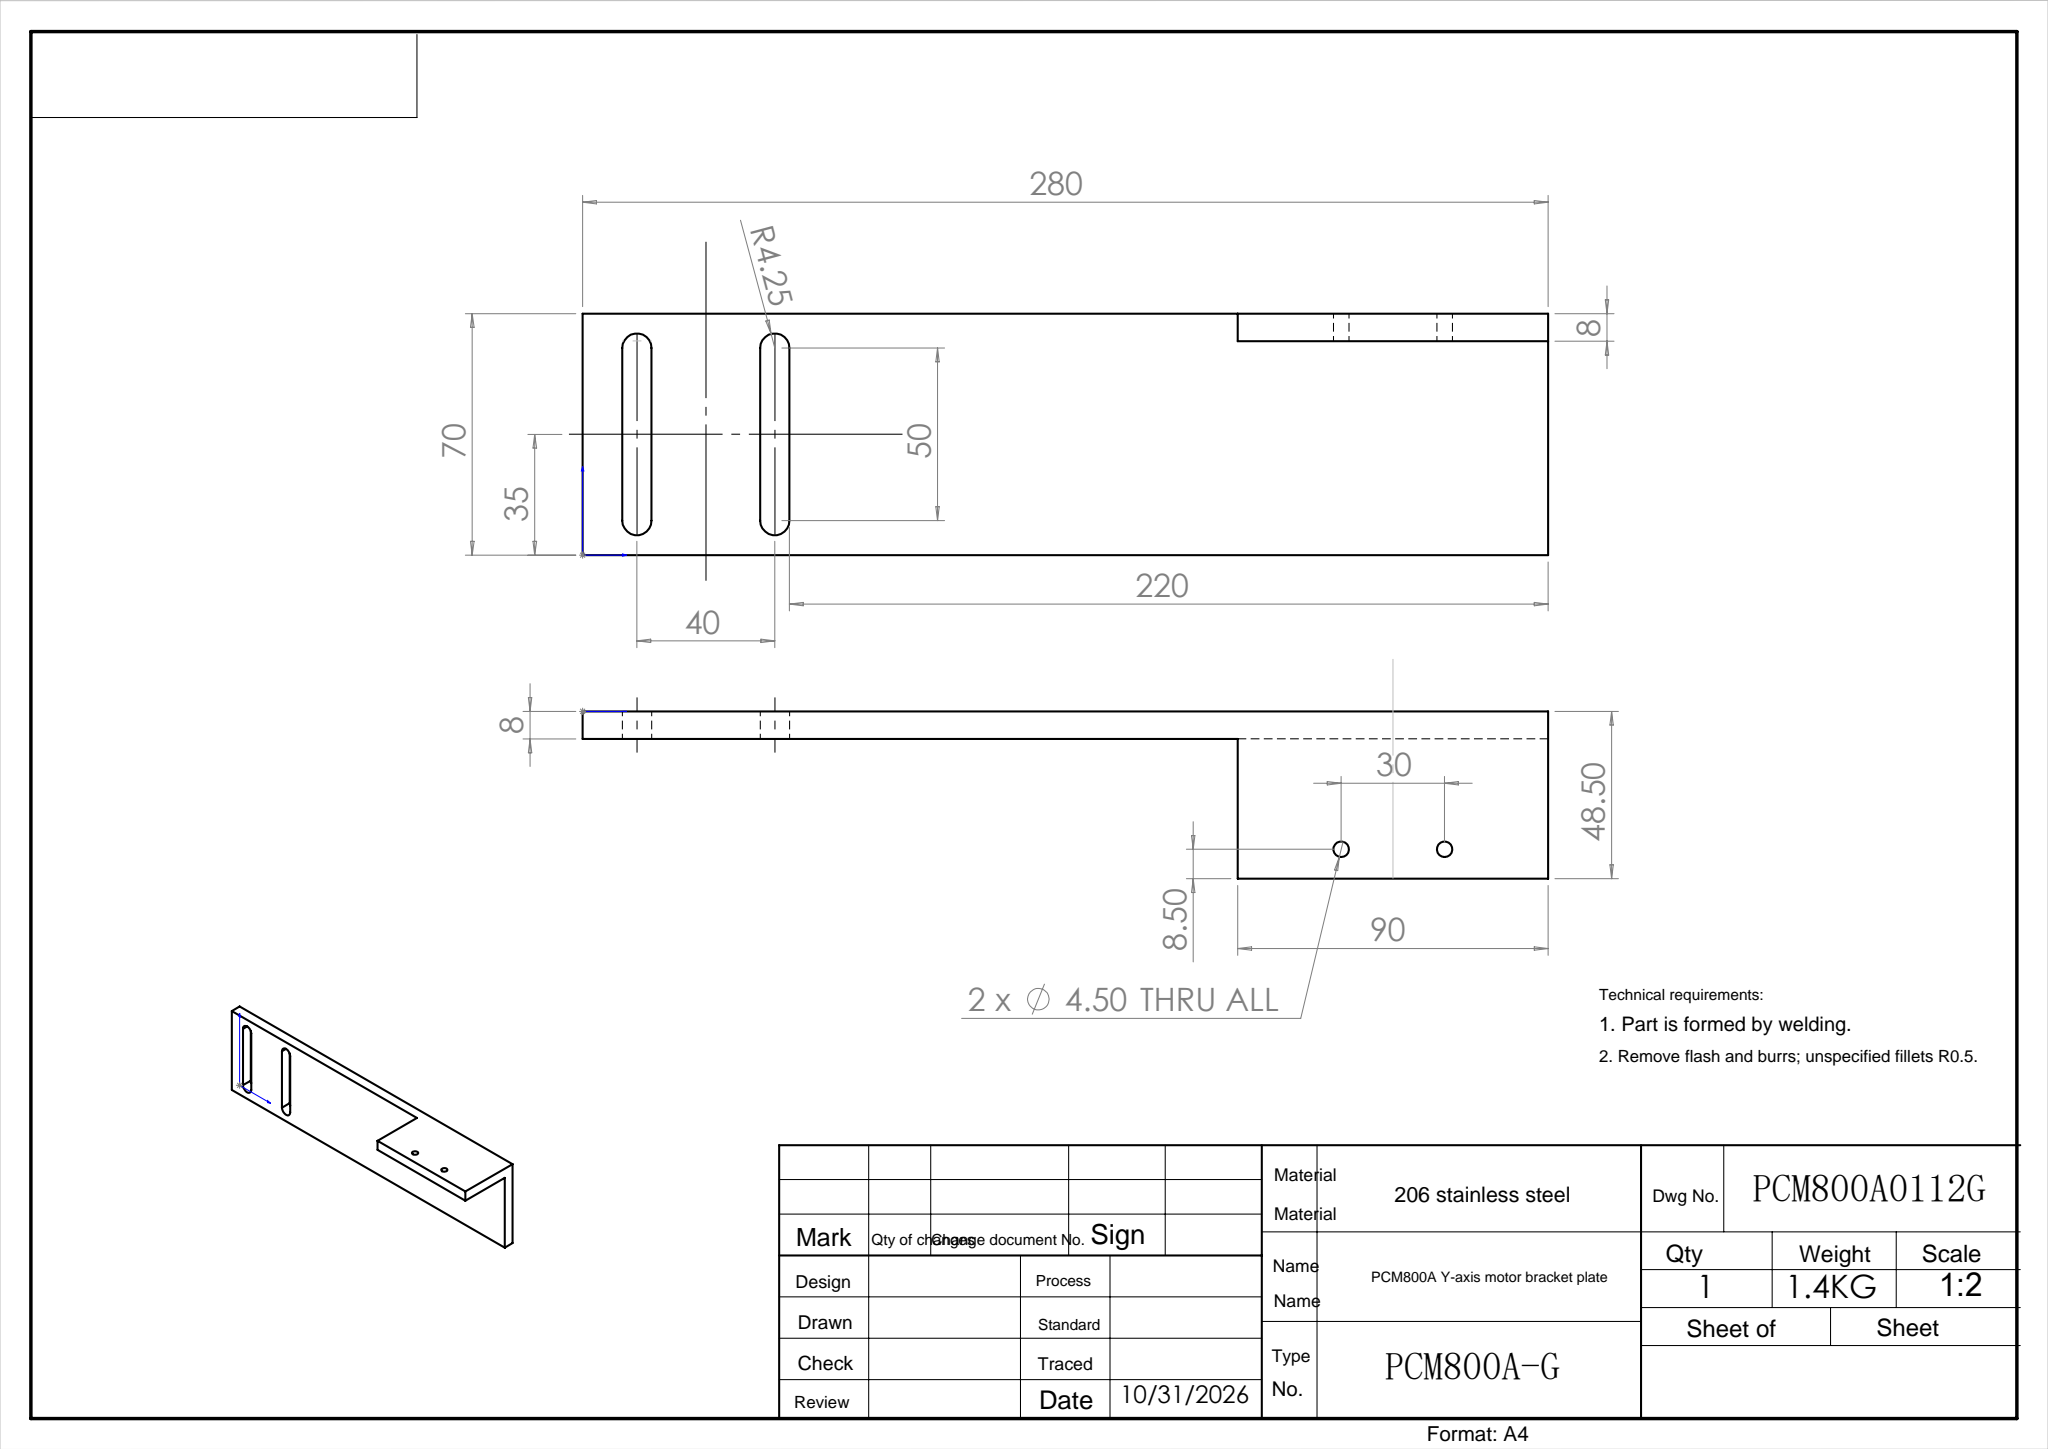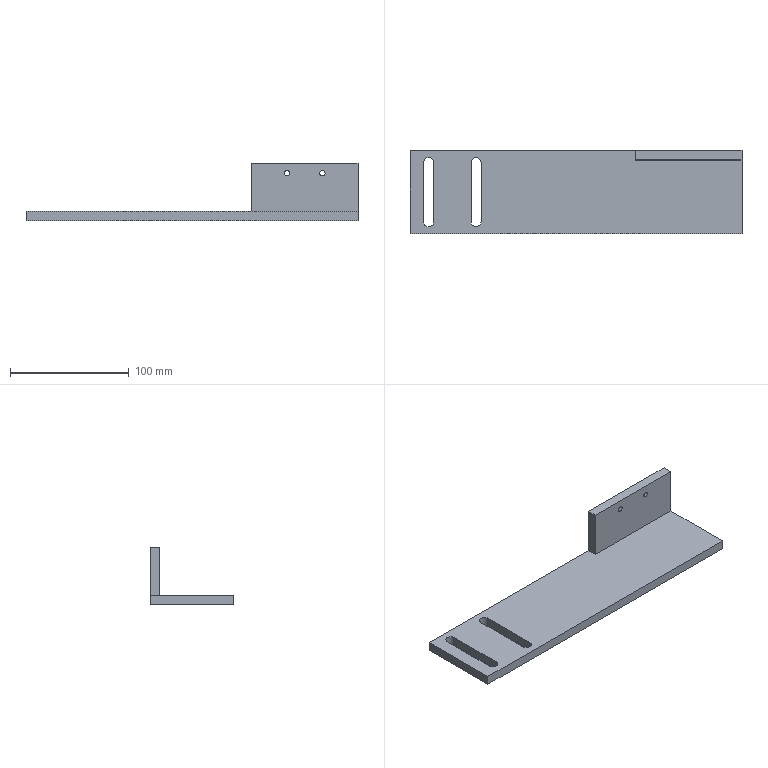Part | SolidWorks | features Extrusion 1, HoleWzd 1, ICE 1 | 1 solid | 21 faces | box 280 x 70 x 48.5 mm | volume 177998 mm3 | plane 13 | cylinder 8 | commonest cylinder face diameters 4.5 x4 8.5 x4
STEP:
#1=CARTESIAN_POINT('',(220.,62.,37.75));
#2=VERTEX_POINT('',#1);
#3=CARTESIAN_POINT('',(220.,62.,42.25));
#4=VERTEX_POINT('',#3);
#5=CARTESIAN_POINT('',(220.,62.,40.));
#6=DIRECTION('',(0.,1.,0.));
#7=DIRECTION('',(0.,0.,1.));
#8=AXIS2_PLACEMENT_3D('',#5,#6,#7);
#9=CIRCLE('',#8,2.25);
#10=EDGE_CURVE('',#2,#4,#9,.T.);
#11=ORIENTED_EDGE('',*,*,#10,.F.);
#12=CARTESIAN_POINT('',(220.,70.,37.75));
#13=VERTEX_POINT('',#12);
#14=CARTESIAN_POINT('',(220.,70.,37.75));
#15=DIRECTION('',(0.,1.,0.));
#16=VECTOR('',#15,1000.);
#17=LINE('',#14,#16);
#18=EDGE_CURVE('',#2,#13,#17,.T.);
#19=ORIENTED_EDGE('',*,*,#18,.T.);
#20=CARTESIAN_POINT('',(220.,70.,42.25));
#21=VERTEX_POINT('',#20);
#22=CARTESIAN_POINT('',(220.,70.,40.));
#23=DIRECTION('',(0.,1.,0.));
#24=DIRECTION('',(0.,0.,1.));
#25=AXIS2_PLACEMENT_3D('',#22,#23,#24);
#26=CIRCLE('',#25,2.25);
#27=EDGE_CURVE('',#13,#21,#26,.T.);
#28=ORIENTED_EDGE('',*,*,#27,.T.);
#29=CARTESIAN_POINT('',(220.,70.,42.25));
#30=DIRECTION('',(0.,1.,0.));
#31=VECTOR('',#30,1000.);
#32=LINE('',#29,#31);
#33=EDGE_CURVE('',#4,#21,#32,.T.);
#34=ORIENTED_EDGE('',*,*,#33,.F.);
#35=EDGE_LOOP('',(#11,#19,#28,#34));
#36=FACE_OUTER_BOUND('',#35,.T.);
#37=CARTESIAN_POINT('',(220.,70.,40.));
#38=DIRECTION('',(0.,1.,0.));
#39=DIRECTION('',(0.,0.,1.));
#40=AXIS2_PLACEMENT_3D('',#37,#38,#39);
#41=CYLINDRICAL_SURFACE('',#40,2.25);
#42=ADVANCED_FACE('',(#36),#41,.F.);
#43=CARTESIAN_POINT('',(250.,62.,37.75));
#44=VERTEX_POINT('',#43);
#45=CARTESIAN_POINT('',(250.,62.,42.25));
#46=VERTEX_POINT('',#45);
#47=CARTESIAN_POINT('',(250.,62.,40.));
#48=DIRECTION('',(0.,1.,0.));
#49=DIRECTION('',(0.,0.,1.));
#50=AXIS2_PLACEMENT_3D('',#47,#48,#49);
#51=CIRCLE('',#50,2.25);
#52=EDGE_CURVE('',#44,#46,#51,.T.);
#53=ORIENTED_EDGE('',*,*,#52,.F.);
#54=CARTESIAN_POINT('',(250.,70.,37.75));
#55=VERTEX_POINT('',#54);
#56=CARTESIAN_POINT('',(250.,70.,37.75));
#57=DIRECTION('',(0.,1.,0.));
#58=VECTOR('',#57,1000.);
#59=LINE('',#56,#58);
#60=EDGE_CURVE('',#44,#55,#59,.T.);
#61=ORIENTED_EDGE('',*,*,#60,.T.);
#62=CARTESIAN_POINT('',(250.,70.,42.25));
#63=VERTEX_POINT('',#62);
#64=CARTESIAN_POINT('',(250.,70.,40.));
#65=DIRECTION('',(0.,1.,0.));
#66=DIRECTION('',(0.,0.,1.));
#67=AXIS2_PLACEMENT_3D('',#64,#65,#66);
#68=CIRCLE('',#67,2.25);
#69=EDGE_CURVE('',#55,#63,#68,.T.);
#70=ORIENTED_EDGE('',*,*,#69,.T.);
#71=CARTESIAN_POINT('',(250.,70.,42.25));
#72=DIRECTION('',(0.,1.,0.));
#73=VECTOR('',#72,1000.);
#74=LINE('',#71,#73);
#75=EDGE_CURVE('',#46,#63,#74,.T.);
#76=ORIENTED_EDGE('',*,*,#75,.F.);
#77=EDGE_LOOP('',(#53,#61,#70,#76));
#78=FACE_OUTER_BOUND('',#77,.T.);
#79=CARTESIAN_POINT('',(250.,70.,40.));
#80=DIRECTION('',(0.,1.,0.));
#81=DIRECTION('',(0.,0.,1.));
#82=AXIS2_PLACEMENT_3D('',#79,#80,#81);
#83=CYLINDRICAL_SURFACE('',#82,2.25);
#84=ADVANCED_FACE('',(#78),#83,.F.);
#85=CARTESIAN_POINT('',(11.5,10.,8.));
#86=VERTEX_POINT('',#85);
#87=CARTESIAN_POINT('',(20.,10.,8.));
#88=VERTEX_POINT('',#87);
#89=CARTESIAN_POINT('',(15.75,10.,8.));
#90=DIRECTION('',(0.,0.,1.));
#91=DIRECTION('',(-1.,0.,0.));
#92=AXIS2_PLACEMENT_3D('',#89,#90,#91);
#93=CIRCLE('',#92,4.25);
#94=EDGE_CURVE('',#86,#88,#93,.T.);
#95=ORIENTED_EDGE('',*,*,#94,.F.);
#96=CARTESIAN_POINT('',(11.5,60.,8.));
#97=VERTEX_POINT('',#96);
#98=CARTESIAN_POINT('',(11.5,60.,8.));
#99=DIRECTION('',(0.,-1.,0.));
#100=VECTOR('',#99,1000.);
#101=LINE('',#98,#100);
#102=EDGE_CURVE('',#97,#86,#101,.T.);
#103=ORIENTED_EDGE('',*,*,#102,.F.);
#104=CARTESIAN_POINT('',(20.,60.,8.));
#105=VERTEX_POINT('',#104);
#106=CARTESIAN_POINT('',(15.75,60.,8.));
#107=DIRECTION('',(0.,0.,1.));
#108=DIRECTION('',(-1.,0.,0.));
#109=AXIS2_PLACEMENT_3D('',#106,#107,#108);
#110=CIRCLE('',#109,4.25);
#111=EDGE_CURVE('',#105,#97,#110,.T.);
#112=ORIENTED_EDGE('',*,*,#111,.F.);
#113=CARTESIAN_POINT('',(20.,60.,8.));
#114=DIRECTION('',(0.,1.,0.));
#115=VECTOR('',#114,1000.);
#116=LINE('',#113,#115);
#117=EDGE_CURVE('',#88,#105,#116,.T.);
#118=ORIENTED_EDGE('',*,*,#117,.F.);
#119=EDGE_LOOP('',(#95,#103,#112,#118));
#120=FACE_BOUND('',#119,.T.);
#121=CARTESIAN_POINT('',(60.,60.,8.));
#122=VERTEX_POINT('',#121);
#123=CARTESIAN_POINT('',(51.5,60.,8.));
#124=VERTEX_POINT('',#123);
#125=CARTESIAN_POINT('',(55.75,60.,8.));
#126=DIRECTION('',(0.,0.,1.));
#127=DIRECTION('',(1.,0.,0.));
#128=AXIS2_PLACEMENT_3D('',#125,#126,#127);
#129=CIRCLE('',#128,4.25);
#130=EDGE_CURVE('',#122,#124,#129,.T.);
#131=ORIENTED_EDGE('',*,*,#130,.F.);
#132=CARTESIAN_POINT('',(60.,10.,8.));
#133=VERTEX_POINT('',#132);
#134=CARTESIAN_POINT('',(60.,60.,8.));
#135=DIRECTION('',(0.,1.,0.));
#136=VECTOR('',#135,1000.);
#137=LINE('',#134,#136);
#138=EDGE_CURVE('',#133,#122,#137,.T.);
#139=ORIENTED_EDGE('',*,*,#138,.F.);
#140=CARTESIAN_POINT('',(51.5,10.,8.));
#141=VERTEX_POINT('',#140);
#142=CARTESIAN_POINT('',(55.75,10.,8.));
#143=DIRECTION('',(0.,0.,1.));
#144=DIRECTION('',(1.,0.,0.));
#145=AXIS2_PLACEMENT_3D('',#142,#143,#144);
#146=CIRCLE('',#145,4.25);
#147=EDGE_CURVE('',#141,#133,#146,.T.);
#148=ORIENTED_EDGE('',*,*,#147,.F.);
#149=CARTESIAN_POINT('',(51.5,60.,8.));
#150=DIRECTION('',(0.,-1.,0.));
#151=VECTOR('',#150,1000.);
#152=LINE('',#149,#151);
#153=EDGE_CURVE('',#124,#141,#152,.T.);
#154=ORIENTED_EDGE('',*,*,#153,.F.);
#155=EDGE_LOOP('',(#131,#139,#148,#154));
#156=FACE_BOUND('',#155,.T.);
#157=CARTESIAN_POINT('',(190.,62.,8.));
#158=VERTEX_POINT('',#157);
#159=CARTESIAN_POINT('',(280.,62.,8.));
#160=VERTEX_POINT('',#159);
#161=CARTESIAN_POINT('',(280.,62.,8.));
#162=DIRECTION('',(1.,0.,0.));
#163=VECTOR('',#162,1000.);
#164=LINE('',#161,#163);
#165=EDGE_CURVE('',#158,#160,#164,.T.);
#166=ORIENTED_EDGE('',*,*,#165,.F.);
#167=CARTESIAN_POINT('',(190.,70.,8.));
#168=VERTEX_POINT('',#167);
#169=CARTESIAN_POINT('',(190.,70.,8.));
#170=DIRECTION('',(0.,-1.,0.));
#171=VECTOR('',#170,1000.);
#172=LINE('',#169,#171);
#173=EDGE_CURVE('',#168,#158,#172,.T.);
#174=ORIENTED_EDGE('',*,*,#173,.F.);
#175=CARTESIAN_POINT('',(0.,70.,8.));
#176=VERTEX_POINT('',#175);
#177=CARTESIAN_POINT('',(0.,70.,8.));
#178=DIRECTION('',(-1.,0.,0.));
#179=VECTOR('',#178,1000.);
#180=LINE('',#177,#179);
#181=EDGE_CURVE('',#168,#176,#180,.T.);
#182=ORIENTED_EDGE('',*,*,#181,.T.);
#183=CARTESIAN_POINT('',(0.,0.,8.));
#184=VERTEX_POINT('',#183);
#185=CARTESIAN_POINT('',(0.,0.,8.));
#186=DIRECTION('',(0.,-1.,0.));
#187=VECTOR('',#186,1000.);
#188=LINE('',#185,#187);
#189=EDGE_CURVE('',#176,#184,#188,.T.);
#190=ORIENTED_EDGE('',*,*,#189,.T.);
#191=CARTESIAN_POINT('',(280.,0.,8.));
#192=VERTEX_POINT('',#191);
#193=CARTESIAN_POINT('',(0.,0.,8.));
#194=DIRECTION('',(1.,0.,0.));
#195=VECTOR('',#194,1000.);
#196=LINE('',#193,#195);
#197=EDGE_CURVE('',#184,#192,#196,.T.);
#198=ORIENTED_EDGE('',*,*,#197,.T.);
#199=CARTESIAN_POINT('',(280.,0.,8.));
#200=DIRECTION('',(0.,1.,0.));
#201=VECTOR('',#200,1000.);
#202=LINE('',#199,#201);
#203=EDGE_CURVE('',#192,#160,#202,.T.);
#204=ORIENTED_EDGE('',*,*,#203,.T.);
#205=EDGE_LOOP('',(#166,#174,#182,#190,#198,#204));
#206=FACE_OUTER_BOUND('',#205,.T.);
#207=CARTESIAN_POINT('',(0.,70.,8.));
#208=DIRECTION('',(0.,0.,-1.));
#209=DIRECTION('',(-1.,0.,0.));
#210=AXIS2_PLACEMENT_3D('',#207,#208,#209);
#211=PLANE('',#210);
#212=ADVANCED_FACE('',(#120,#156,#206),#211,.F.);
#213=CARTESIAN_POINT('',(60.,10.,0.));
#214=VERTEX_POINT('',#213);
#215=CARTESIAN_POINT('',(60.,60.,0.));
#216=VERTEX_POINT('',#215);
#217=CARTESIAN_POINT('',(60.,60.,0.));
#218=DIRECTION('',(0.,1.,0.));
#219=VECTOR('',#218,1000.);
#220=LINE('',#217,#219);
#221=EDGE_CURVE('',#214,#216,#220,.T.);
#222=ORIENTED_EDGE('',*,*,#221,.T.);
#223=CARTESIAN_POINT('',(51.5,60.,0.));
#224=VERTEX_POINT('',#223);
#225=CARTESIAN_POINT('',(55.75,60.,0.));
#226=DIRECTION('',(0.,0.,1.));
#227=DIRECTION('',(1.,0.,0.));
#228=AXIS2_PLACEMENT_3D('',#225,#226,#227);
#229=CIRCLE('',#228,4.25);
#230=EDGE_CURVE('',#216,#224,#229,.T.);
#231=ORIENTED_EDGE('',*,*,#230,.T.);
#232=CARTESIAN_POINT('',(51.5,10.,0.));
#233=VERTEX_POINT('',#232);
#234=CARTESIAN_POINT('',(51.5,60.,0.));
#235=DIRECTION('',(0.,-1.,0.));
#236=VECTOR('',#235,1000.);
#237=LINE('',#234,#236);
#238=EDGE_CURVE('',#224,#233,#237,.T.);
#239=ORIENTED_EDGE('',*,*,#238,.T.);
#240=CARTESIAN_POINT('',(55.75,10.,0.));
#241=DIRECTION('',(0.,0.,1.));
#242=DIRECTION('',(1.,0.,0.));
#243=AXIS2_PLACEMENT_3D('',#240,#241,#242);
#244=CIRCLE('',#243,4.25);
#245=EDGE_CURVE('',#233,#214,#244,.T.);
#246=ORIENTED_EDGE('',*,*,#245,.T.);
#247=EDGE_LOOP('',(#222,#231,#239,#246));
#248=FACE_BOUND('',#247,.T.);
#249=CARTESIAN_POINT('',(0.,70.,0.));
#250=VERTEX_POINT('',#249);
#251=CARTESIAN_POINT('',(0.,0.,0.));
#252=VERTEX_POINT('',#251);
#253=CARTESIAN_POINT('',(0.,0.,0.));
#254=DIRECTION('',(0.,-1.,0.));
#255=VECTOR('',#254,1000.);
#256=LINE('',#253,#255);
#257=EDGE_CURVE('',#250,#252,#256,.T.);
#258=ORIENTED_EDGE('',*,*,#257,.F.);
#259=CARTESIAN_POINT('',(280.,70.,0.));
#260=VERTEX_POINT('',#259);
#261=CARTESIAN_POINT('',(0.,70.,0.));
#262=DIRECTION('',(-1.,0.,0.));
#263=VECTOR('',#262,1000.);
#264=LINE('',#261,#263);
#265=EDGE_CURVE('',#260,#250,#264,.T.);
#266=ORIENTED_EDGE('',*,*,#265,.F.);
#267=CARTESIAN_POINT('',(280.,0.,0.));
#268=VERTEX_POINT('',#267);
#269=CARTESIAN_POINT('',(280.,0.,0.));
#270=DIRECTION('',(0.,1.,0.));
#271=VECTOR('',#270,1000.);
#272=LINE('',#269,#271);
#273=EDGE_CURVE('',#268,#260,#272,.T.);
#274=ORIENTED_EDGE('',*,*,#273,.F.);
#275=CARTESIAN_POINT('',(0.,0.,0.));
#276=DIRECTION('',(1.,0.,0.));
#277=VECTOR('',#276,1000.);
#278=LINE('',#275,#277);
#279=EDGE_CURVE('',#252,#268,#278,.T.);
#280=ORIENTED_EDGE('',*,*,#279,.F.);
#281=EDGE_LOOP('',(#258,#266,#274,#280));
#282=FACE_OUTER_BOUND('',#281,.T.);
#283=CARTESIAN_POINT('',(11.5,60.,0.));
#284=VERTEX_POINT('',#283);
#285=CARTESIAN_POINT('',(11.5,10.,0.));
#286=VERTEX_POINT('',#285);
#287=CARTESIAN_POINT('',(11.5,60.,0.));
#288=DIRECTION('',(0.,-1.,0.));
#289=VECTOR('',#288,1000.);
#290=LINE('',#287,#289);
#291=EDGE_CURVE('',#284,#286,#290,.T.);
#292=ORIENTED_EDGE('',*,*,#291,.T.);
#293=CARTESIAN_POINT('',(20.,10.,0.));
#294=VERTEX_POINT('',#293);
#295=CARTESIAN_POINT('',(15.75,10.,0.));
#296=DIRECTION('',(0.,0.,1.));
#297=DIRECTION('',(-1.,0.,0.));
#298=AXIS2_PLACEMENT_3D('',#295,#296,#297);
#299=CIRCLE('',#298,4.25);
#300=EDGE_CURVE('',#286,#294,#299,.T.);
#301=ORIENTED_EDGE('',*,*,#300,.T.);
#302=CARTESIAN_POINT('',(20.,60.,0.));
#303=VERTEX_POINT('',#302);
#304=CARTESIAN_POINT('',(20.,60.,0.));
#305=DIRECTION('',(0.,1.,0.));
#306=VECTOR('',#305,1000.);
#307=LINE('',#304,#306);
#308=EDGE_CURVE('',#294,#303,#307,.T.);
#309=ORIENTED_EDGE('',*,*,#308,.T.);
#310=CARTESIAN_POINT('',(15.75,60.,0.));
#311=DIRECTION('',(0.,0.,1.));
#312=DIRECTION('',(-1.,0.,0.));
#313=AXIS2_PLACEMENT_3D('',#310,#311,#312);
#314=CIRCLE('',#313,4.25);
#315=EDGE_CURVE('',#303,#284,#314,.T.);
#316=ORIENTED_EDGE('',*,*,#315,.T.);
#317=EDGE_LOOP('',(#292,#301,#309,#316));
#318=FACE_BOUND('',#317,.T.);
#319=CARTESIAN_POINT('',(0.,70.,0.));
#320=DIRECTION('',(0.,0.,-1.));
#321=DIRECTION('',(-1.,0.,0.));
#322=AXIS2_PLACEMENT_3D('',#319,#320,#321);
#323=PLANE('',#322);
#324=ADVANCED_FACE('',(#248,#282,#318),#323,.T.);
#325=ORIENTED_EDGE('',*,*,#257,.T.);
#326=CARTESIAN_POINT('',(0.,0.,8.));
#327=DIRECTION('',(0.,0.,-1.));
#328=VECTOR('',#327,1000.);
#329=LINE('',#326,#328);
#330=EDGE_CURVE('',#184,#252,#329,.T.);
#331=ORIENTED_EDGE('',*,*,#330,.F.);
#332=ORIENTED_EDGE('',*,*,#189,.F.);
#333=CARTESIAN_POINT('',(0.,70.,8.));
#334=DIRECTION('',(0.,0.,-1.));
#335=VECTOR('',#334,1000.);
#336=LINE('',#333,#335);
#337=EDGE_CURVE('',#176,#250,#336,.T.);
#338=ORIENTED_EDGE('',*,*,#337,.T.);
#339=EDGE_LOOP('',(#325,#331,#332,#338));
#340=FACE_OUTER_BOUND('',#339,.T.);
#341=CARTESIAN_POINT('',(0.,0.,8.));
#342=DIRECTION('',(1.,0.,0.));
#343=DIRECTION('',(0.,0.,-1.));
#344=AXIS2_PLACEMENT_3D('',#341,#342,#343);
#345=PLANE('',#344);
#346=ADVANCED_FACE('',(#340),#345,.F.);
#347=ORIENTED_EDGE('',*,*,#279,.T.);
#348=CARTESIAN_POINT('',(280.,0.,8.));
#349=DIRECTION('',(0.,0.,-1.));
#350=VECTOR('',#349,1000.);
#351=LINE('',#348,#350);
#352=EDGE_CURVE('',#192,#268,#351,.T.);
#353=ORIENTED_EDGE('',*,*,#352,.F.);
#354=ORIENTED_EDGE('',*,*,#197,.F.);
#355=ORIENTED_EDGE('',*,*,#330,.T.);
#356=EDGE_LOOP('',(#347,#353,#354,#355));
#357=FACE_OUTER_BOUND('',#356,.T.);
#358=CARTESIAN_POINT('',(0.,0.,8.));
#359=DIRECTION('',(0.,1.,0.));
#360=DIRECTION('',(0.,0.,1.));
#361=AXIS2_PLACEMENT_3D('',#358,#359,#360);
#362=PLANE('',#361);
#363=ADVANCED_FACE('',(#357),#362,.F.);
#364=ORIENTED_EDGE('',*,*,#273,.T.);
#365=CARTESIAN_POINT('',(280.,70.,48.5));
#366=VERTEX_POINT('',#365);
#367=CARTESIAN_POINT('',(280.,70.,8.));
#368=DIRECTION('',(0.,0.,-1.));
#369=VECTOR('',#368,1000.);
#370=LINE('',#367,#369);
#371=EDGE_CURVE('',#366,#260,#370,.T.);
#372=ORIENTED_EDGE('',*,*,#371,.F.);
#373=CARTESIAN_POINT('',(280.,62.,48.5));
#374=VERTEX_POINT('',#373);
#375=CARTESIAN_POINT('',(280.,70.,48.5));
#376=DIRECTION('',(0.,1.,0.));
#377=VECTOR('',#376,1000.);
#378=LINE('',#375,#377);
#379=EDGE_CURVE('',#374,#366,#378,.T.);
#380=ORIENTED_EDGE('',*,*,#379,.F.);
#381=CARTESIAN_POINT('',(280.,62.,48.5));
#382=DIRECTION('',(0.,0.,-1.));
#383=VECTOR('',#382,1000.);
#384=LINE('',#381,#383);
#385=EDGE_CURVE('',#374,#160,#384,.T.);
#386=ORIENTED_EDGE('',*,*,#385,.T.);
#387=ORIENTED_EDGE('',*,*,#203,.F.);
#388=ORIENTED_EDGE('',*,*,#352,.T.);
#389=EDGE_LOOP('',(#364,#372,#380,#386,#387,#388));
#390=FACE_OUTER_BOUND('',#389,.T.);
#391=CARTESIAN_POINT('',(280.,0.,8.));
#392=DIRECTION('',(-1.,0.,0.));
#393=DIRECTION('',(0.,0.,1.));
#394=AXIS2_PLACEMENT_3D('',#391,#392,#393);
#395=PLANE('',#394);
#396=ADVANCED_FACE('',(#390),#395,.F.);
#397=CARTESIAN_POINT('',(220.,70.,40.));
#398=DIRECTION('',(0.,1.,0.));
#399=DIRECTION('',(0.,0.,1.));
#400=AXIS2_PLACEMENT_3D('',#397,#398,#399);
#401=CIRCLE('',#400,2.25);
#402=EDGE_CURVE('',#21,#13,#401,.T.);
#403=ORIENTED_EDGE('',*,*,#402,.F.);
#404=ORIENTED_EDGE('',*,*,#27,.F.);
#405=EDGE_LOOP('',(#403,#404));
#406=FACE_BOUND('',#405,.T.);
#407=CARTESIAN_POINT('',(250.,70.,40.));
#408=DIRECTION('',(0.,1.,0.));
#409=DIRECTION('',(0.,0.,1.));
#410=AXIS2_PLACEMENT_3D('',#407,#408,#409);
#411=CIRCLE('',#410,2.25);
#412=EDGE_CURVE('',#63,#55,#411,.T.);
#413=ORIENTED_EDGE('',*,*,#412,.F.);
#414=ORIENTED_EDGE('',*,*,#69,.F.);
#415=EDGE_LOOP('',(#413,#414));
#416=FACE_BOUND('',#415,.T.);
#417=ORIENTED_EDGE('',*,*,#265,.T.);
#418=ORIENTED_EDGE('',*,*,#337,.F.);
#419=ORIENTED_EDGE('',*,*,#181,.F.);
#420=CARTESIAN_POINT('',(190.,70.,48.5));
#421=VERTEX_POINT('',#420);
#422=CARTESIAN_POINT('',(190.,70.,48.5));
#423=DIRECTION('',(0.,0.,-1.));
#424=VECTOR('',#423,1000.);
#425=LINE('',#422,#424);
#426=EDGE_CURVE('',#421,#168,#425,.T.);
#427=ORIENTED_EDGE('',*,*,#426,.F.);
#428=CARTESIAN_POINT('',(280.,70.,48.5));
#429=DIRECTION('',(-1.,0.,0.));
#430=VECTOR('',#429,1000.);
#431=LINE('',#428,#430);
#432=EDGE_CURVE('',#366,#421,#431,.T.);
#433=ORIENTED_EDGE('',*,*,#432,.F.);
#434=ORIENTED_EDGE('',*,*,#371,.T.);
#435=EDGE_LOOP('',(#417,#418,#419,#427,#433,#434));
#436=FACE_OUTER_BOUND('',#435,.T.);
#437=CARTESIAN_POINT('',(0.,70.,8.));
#438=DIRECTION('',(0.,-1.,0.));
#439=DIRECTION('',(0.,0.,-1.));
#440=AXIS2_PLACEMENT_3D('',#437,#438,#439);
#441=PLANE('',#440);
#442=ADVANCED_FACE('',(#406,#416,#436),#441,.F.);
#443=ORIENTED_EDGE('',*,*,#230,.F.);
#444=CARTESIAN_POINT('',(60.,60.,8.));
#445=DIRECTION('',(0.,0.,-1.));
#446=VECTOR('',#445,1000.);
#447=LINE('',#444,#446);
#448=EDGE_CURVE('',#122,#216,#447,.T.);
#449=ORIENTED_EDGE('',*,*,#448,.F.);
#450=ORIENTED_EDGE('',*,*,#130,.T.);
#451=CARTESIAN_POINT('',(51.5,60.,8.));
#452=DIRECTION('',(0.,0.,-1.));
#453=VECTOR('',#452,1000.);
#454=LINE('',#451,#453);
#455=EDGE_CURVE('',#124,#224,#454,.T.);
#456=ORIENTED_EDGE('',*,*,#455,.T.);
#457=EDGE_LOOP('',(#443,#449,#450,#456));
#458=FACE_OUTER_BOUND('',#457,.T.);
#459=CARTESIAN_POINT('',(55.75,60.,8.));
#460=DIRECTION('',(0.,0.,-1.));
#461=DIRECTION('',(-1.,0.,0.));
#462=AXIS2_PLACEMENT_3D('',#459,#460,#461);
#463=CYLINDRICAL_SURFACE('',#462,4.25);
#464=ADVANCED_FACE('',(#458),#463,.F.);
#465=ORIENTED_EDGE('',*,*,#238,.F.);
#466=ORIENTED_EDGE('',*,*,#455,.F.);
#467=ORIENTED_EDGE('',*,*,#153,.T.);
#468=CARTESIAN_POINT('',(51.5,10.,8.));
#469=DIRECTION('',(0.,0.,-1.));
#470=VECTOR('',#469,1000.);
#471=LINE('',#468,#470);
#472=EDGE_CURVE('',#141,#233,#471,.T.);
#473=ORIENTED_EDGE('',*,*,#472,.T.);
#474=EDGE_LOOP('',(#465,#466,#467,#473));
#475=FACE_OUTER_BOUND('',#474,.T.);
#476=CARTESIAN_POINT('',(51.5,60.,8.));
#477=DIRECTION('',(1.,0.,0.));
#478=DIRECTION('',(0.,1.,0.));
#479=AXIS2_PLACEMENT_3D('',#476,#477,#478);
#480=PLANE('',#479);
#481=ADVANCED_FACE('',(#475),#480,.T.);
#482=ORIENTED_EDGE('',*,*,#245,.F.);
#483=ORIENTED_EDGE('',*,*,#472,.F.);
#484=ORIENTED_EDGE('',*,*,#147,.T.);
#485=CARTESIAN_POINT('',(60.,10.,8.));
#486=DIRECTION('',(0.,0.,-1.));
#487=VECTOR('',#486,1000.);
#488=LINE('',#485,#487);
#489=EDGE_CURVE('',#133,#214,#488,.T.);
#490=ORIENTED_EDGE('',*,*,#489,.T.);
#491=EDGE_LOOP('',(#482,#483,#484,#490));
#492=FACE_OUTER_BOUND('',#491,.T.);
#493=CARTESIAN_POINT('',(55.75,10.,8.));
#494=DIRECTION('',(0.,0.,-1.));
#495=DIRECTION('',(-1.,0.,0.));
#496=AXIS2_PLACEMENT_3D('',#493,#494,#495);
#497=CYLINDRICAL_SURFACE('',#496,4.25);
#498=ADVANCED_FACE('',(#492),#497,.F.);
#499=ORIENTED_EDGE('',*,*,#221,.F.);
#500=ORIENTED_EDGE('',*,*,#489,.F.);
#501=ORIENTED_EDGE('',*,*,#138,.T.);
#502=ORIENTED_EDGE('',*,*,#448,.T.);
#503=EDGE_LOOP('',(#499,#500,#501,#502));
#504=FACE_OUTER_BOUND('',#503,.T.);
#505=CARTESIAN_POINT('',(60.,60.,8.));
#506=DIRECTION('',(-1.,0.,0.));
#507=DIRECTION('',(0.,-1.,0.));
#508=AXIS2_PLACEMENT_3D('',#505,#506,#507);
#509=PLANE('',#508);
#510=ADVANCED_FACE('',(#504),#509,.T.);
#511=ORIENTED_EDGE('',*,*,#300,.F.);
#512=CARTESIAN_POINT('',(11.5,10.,8.));
#513=DIRECTION('',(0.,0.,-1.));
#514=VECTOR('',#513,1000.);
#515=LINE('',#512,#514);
#516=EDGE_CURVE('',#86,#286,#515,.T.);
#517=ORIENTED_EDGE('',*,*,#516,.F.);
#518=ORIENTED_EDGE('',*,*,#94,.T.);
#519=CARTESIAN_POINT('',(20.,10.,8.));
#520=DIRECTION('',(0.,0.,-1.));
#521=VECTOR('',#520,1000.);
#522=LINE('',#519,#521);
#523=EDGE_CURVE('',#88,#294,#522,.T.);
#524=ORIENTED_EDGE('',*,*,#523,.T.);
#525=EDGE_LOOP('',(#511,#517,#518,#524));
#526=FACE_OUTER_BOUND('',#525,.T.);
#527=CARTESIAN_POINT('',(15.75,10.,8.));
#528=DIRECTION('',(0.,0.,-1.));
#529=DIRECTION('',(-1.,0.,0.));
#530=AXIS2_PLACEMENT_3D('',#527,#528,#529);
#531=CYLINDRICAL_SURFACE('',#530,4.25);
#532=ADVANCED_FACE('',(#526),#531,.F.);
#533=ORIENTED_EDGE('',*,*,#308,.F.);
#534=ORIENTED_EDGE('',*,*,#523,.F.);
#535=ORIENTED_EDGE('',*,*,#117,.T.);
#536=CARTESIAN_POINT('',(20.,60.,8.));
#537=DIRECTION('',(0.,0.,-1.));
#538=VECTOR('',#537,1000.);
#539=LINE('',#536,#538);
#540=EDGE_CURVE('',#105,#303,#539,.T.);
#541=ORIENTED_EDGE('',*,*,#540,.T.);
#542=EDGE_LOOP('',(#533,#534,#535,#541));
#543=FACE_OUTER_BOUND('',#542,.T.);
#544=CARTESIAN_POINT('',(20.,60.,8.));
#545=DIRECTION('',(-1.,0.,0.));
#546=DIRECTION('',(0.,0.,1.));
#547=AXIS2_PLACEMENT_3D('',#544,#545,#546);
#548=PLANE('',#547);
#549=ADVANCED_FACE('',(#543),#548,.T.);
#550=ORIENTED_EDGE('',*,*,#315,.F.);
#551=ORIENTED_EDGE('',*,*,#540,.F.);
#552=ORIENTED_EDGE('',*,*,#111,.T.);
#553=CARTESIAN_POINT('',(11.5,60.,8.));
#554=DIRECTION('',(0.,0.,-1.));
#555=VECTOR('',#554,1000.);
#556=LINE('',#553,#555);
#557=EDGE_CURVE('',#97,#284,#556,.T.);
#558=ORIENTED_EDGE('',*,*,#557,.T.);
#559=EDGE_LOOP('',(#550,#551,#552,#558));
#560=FACE_OUTER_BOUND('',#559,.T.);
#561=CARTESIAN_POINT('',(15.75,60.,8.));
#562=DIRECTION('',(0.,0.,-1.));
#563=DIRECTION('',(-1.,0.,0.));
#564=AXIS2_PLACEMENT_3D('',#561,#562,#563);
#565=CYLINDRICAL_SURFACE('',#564,4.25);
#566=ADVANCED_FACE('',(#560),#565,.F.);
#567=ORIENTED_EDGE('',*,*,#291,.F.);
#568=ORIENTED_EDGE('',*,*,#557,.F.);
#569=ORIENTED_EDGE('',*,*,#102,.T.);
#570=ORIENTED_EDGE('',*,*,#516,.T.);
#571=EDGE_LOOP('',(#567,#568,#569,#570));
#572=FACE_OUTER_BOUND('',#571,.T.);
#573=CARTESIAN_POINT('',(11.5,60.,8.));
#574=DIRECTION('',(1.,0.,0.));
#575=DIRECTION('',(0.,1.,0.));
#576=AXIS2_PLACEMENT_3D('',#573,#574,#575);
#577=PLANE('',#576);
#578=ADVANCED_FACE('',(#572),#577,.T.);
#579=ORIENTED_EDGE('',*,*,#173,.T.);
#580=CARTESIAN_POINT('',(190.,62.,48.5));
#581=VERTEX_POINT('',#580);
#582=CARTESIAN_POINT('',(190.,62.,48.5));
#583=DIRECTION('',(0.,0.,-1.));
#584=VECTOR('',#583,1000.);
#585=LINE('',#582,#584);
#586=EDGE_CURVE('',#581,#158,#585,.T.);
#587=ORIENTED_EDGE('',*,*,#586,.F.);
#588=CARTESIAN_POINT('',(190.,70.,48.5));
#589=DIRECTION('',(0.,-1.,0.));
#590=VECTOR('',#589,1000.);
#591=LINE('',#588,#590);
#592=EDGE_CURVE('',#421,#581,#591,.T.);
#593=ORIENTED_EDGE('',*,*,#592,.F.);
#594=ORIENTED_EDGE('',*,*,#426,.T.);
#595=EDGE_LOOP('',(#579,#587,#593,#594));
#596=FACE_OUTER_BOUND('',#595,.T.);
#597=CARTESIAN_POINT('',(190.,70.,48.5));
#598=DIRECTION('',(1.,0.,0.));
#599=DIRECTION('',(0.,0.,-1.));
#600=AXIS2_PLACEMENT_3D('',#597,#598,#599);
#601=PLANE('',#600);
#602=ADVANCED_FACE('',(#596),#601,.F.);
#603=CARTESIAN_POINT('',(220.,62.,40.));
#604=DIRECTION('',(0.,1.,0.));
#605=DIRECTION('',(0.,0.,1.));
#606=AXIS2_PLACEMENT_3D('',#603,#604,#605);
#607=CIRCLE('',#606,2.25);
#608=EDGE_CURVE('',#4,#2,#607,.T.);
#609=ORIENTED_EDGE('',*,*,#608,.T.);
#610=ORIENTED_EDGE('',*,*,#10,.T.);
#611=EDGE_LOOP('',(#609,#610));
#612=FACE_BOUND('',#611,.T.);
#613=CARTESIAN_POINT('',(250.,62.,40.));
#614=DIRECTION('',(0.,1.,0.));
#615=DIRECTION('',(0.,0.,1.));
#616=AXIS2_PLACEMENT_3D('',#613,#614,#615);
#617=CIRCLE('',#616,2.25);
#618=EDGE_CURVE('',#46,#44,#617,.T.);
#619=ORIENTED_EDGE('',*,*,#618,.T.);
#620=ORIENTED_EDGE('',*,*,#52,.T.);
#621=EDGE_LOOP('',(#619,#620));
#622=FACE_BOUND('',#621,.T.);
#623=ORIENTED_EDGE('',*,*,#165,.T.);
#624=ORIENTED_EDGE('',*,*,#385,.F.);
#625=CARTESIAN_POINT('',(280.,62.,48.5));
#626=DIRECTION('',(1.,0.,0.));
#627=VECTOR('',#626,1000.);
#628=LINE('',#625,#627);
#629=EDGE_CURVE('',#581,#374,#628,.T.);
#630=ORIENTED_EDGE('',*,*,#629,.F.);
#631=ORIENTED_EDGE('',*,*,#586,.T.);
#632=EDGE_LOOP('',(#623,#624,#630,#631));
#633=FACE_OUTER_BOUND('',#632,.T.);
#634=CARTESIAN_POINT('',(280.,62.,48.5));
#635=DIRECTION('',(0.,1.,0.));
#636=DIRECTION('',(0.,0.,1.));
#637=AXIS2_PLACEMENT_3D('',#634,#635,#636);
#638=PLANE('',#637);
#639=ADVANCED_FACE('',(#612,#622,#633),#638,.F.);
#640=ORIENTED_EDGE('',*,*,#379,.T.);
#641=ORIENTED_EDGE('',*,*,#432,.T.);
#642=ORIENTED_EDGE('',*,*,#592,.T.);
#643=ORIENTED_EDGE('',*,*,#629,.T.);
#644=EDGE_LOOP('',(#640,#641,#642,#643));
#645=FACE_OUTER_BOUND('',#644,.T.);
#646=CARTESIAN_POINT('',(280.,62.,48.5));
#647=DIRECTION('',(0.,0.,-1.));
#648=DIRECTION('',(-1.,0.,0.));
#649=AXIS2_PLACEMENT_3D('',#646,#647,#648);
#650=PLANE('',#649);
#651=ADVANCED_FACE('',(#645),#650,.F.);
#652=ORIENTED_EDGE('',*,*,#60,.F.);
#653=ORIENTED_EDGE('',*,*,#618,.F.);
#654=ORIENTED_EDGE('',*,*,#75,.T.);
#655=ORIENTED_EDGE('',*,*,#412,.T.);
#656=EDGE_LOOP('',(#652,#653,#654,#655));
#657=FACE_OUTER_BOUND('',#656,.T.);
#658=CARTESIAN_POINT('',(250.,70.,40.));
#659=DIRECTION('',(0.,1.,0.));
#660=DIRECTION('',(0.,0.,1.));
#661=AXIS2_PLACEMENT_3D('',#658,#659,#660);
#662=CYLINDRICAL_SURFACE('',#661,2.25);
#663=ADVANCED_FACE('',(#657),#662,.F.);
#664=ORIENTED_EDGE('',*,*,#18,.F.);
#665=ORIENTED_EDGE('',*,*,#608,.F.);
#666=ORIENTED_EDGE('',*,*,#33,.T.);
#667=ORIENTED_EDGE('',*,*,#402,.T.);
#668=EDGE_LOOP('',(#664,#665,#666,#667));
#669=FACE_OUTER_BOUND('',#668,.T.);
#670=CARTESIAN_POINT('',(220.,70.,40.));
#671=DIRECTION('',(0.,1.,0.));
#672=DIRECTION('',(0.,0.,1.));
#673=AXIS2_PLACEMENT_3D('',#670,#671,#672);
#674=CYLINDRICAL_SURFACE('',#673,2.25);
#675=ADVANCED_FACE('',(#669),#674,.F.);
#676=CLOSED_SHELL('',(#42,#84,#212,#324,#346,#363,#396,#442,#464,#481,#498,#510,#532,#549,#566,#578,#602,#639,#651,#663,#675));
#677=MANIFOLD_SOLID_BREP('',#676);
#678=CARTESIAN_POINT('',(0.,0.,0.));
#679=DIRECTION('',(0.,0.,1.));
#680=DIRECTION('',(1.,0.,0.));
#681=AXIS2_PLACEMENT_3D('',#678,#679,#680);
#682=(LENGTH_UNIT()NAMED_UNIT(*)SI_UNIT(.MILLI.,.METRE.));
#683=UNCERTAINTY_MEASURE_WITH_UNIT(LENGTH_MEASURE(0.00001),#682,'','');
#684=(NAMED_UNIT(*)PLANE_ANGLE_UNIT()SI_UNIT($,.RADIAN.));
#685=(NAMED_UNIT(*)SI_UNIT($,.STERADIAN.)SOLID_ANGLE_UNIT());
#686=(GEOMETRIC_REPRESENTATION_CONTEXT(3)GLOBAL_UNCERTAINTY_ASSIGNED_CONTEXT((#683))GLOBAL_UNIT_ASSIGNED_CONTEXT((#682,#684,#685))REPRESENTATION_CONTEXT('',''));
#687=ADVANCED_BREP_SHAPE_REPRESENTATION('',(#677,#681),#686);